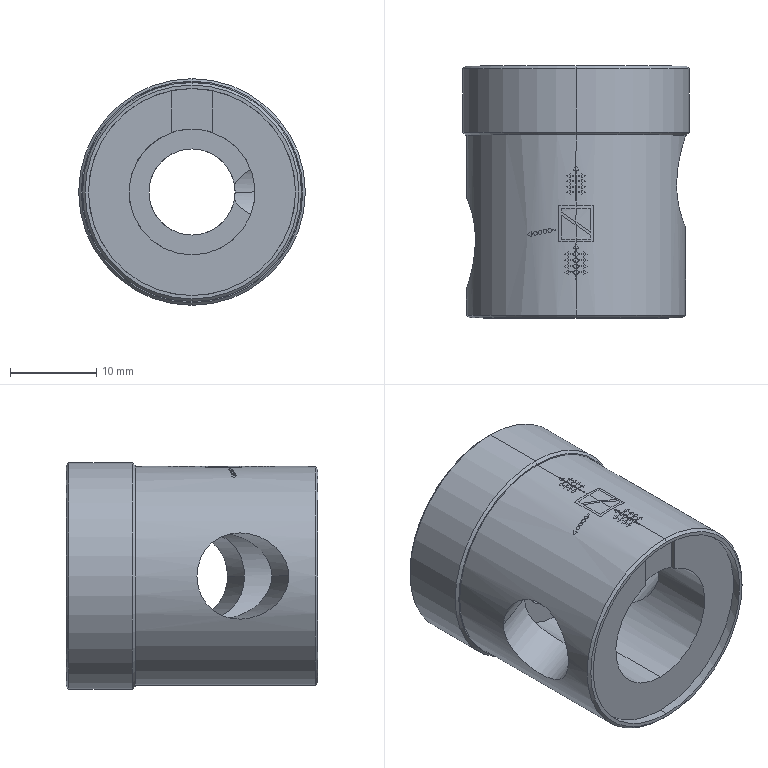Part | STEP file | 1 solid | 46 faces | box 26.29 x 29.2 x 26.29 mm | volume 9926 mm3 | cylinder 25 | plane 15 | cone 6 | commonest cylinder face diameters 25.4 x13 10 x6 14.6 x2 24 x2 26.29 x2